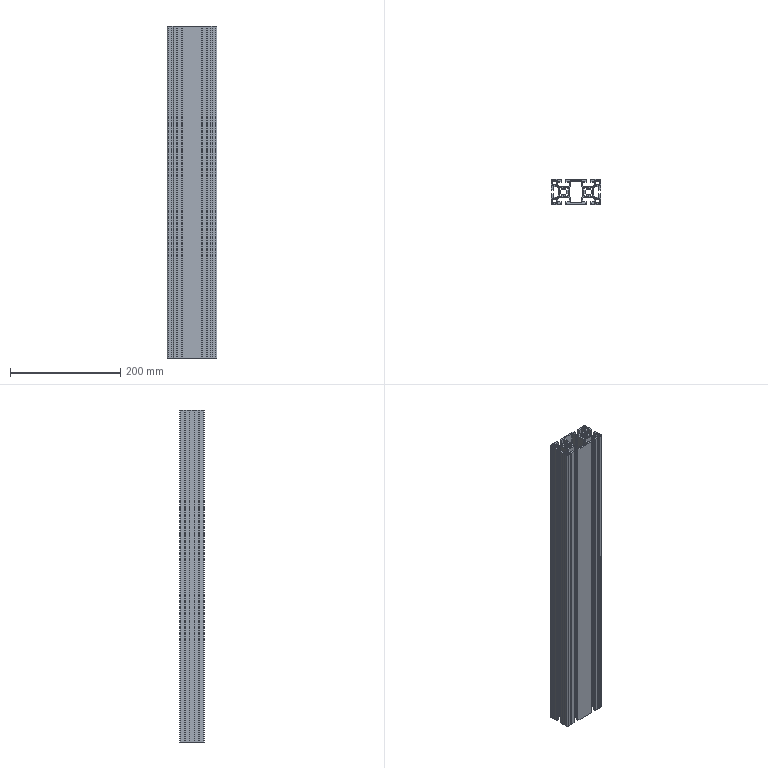Part | STEP file | 4590-705 aluminium profile (rear column 2) | 1 solid | 366 faces | box 90 x 45 x 603 mm | volume 707141 mm3 | plane 254 | cylinder 112 | commonest cylinder face diameters 2 x64 8 x20 12 x16 4 x12